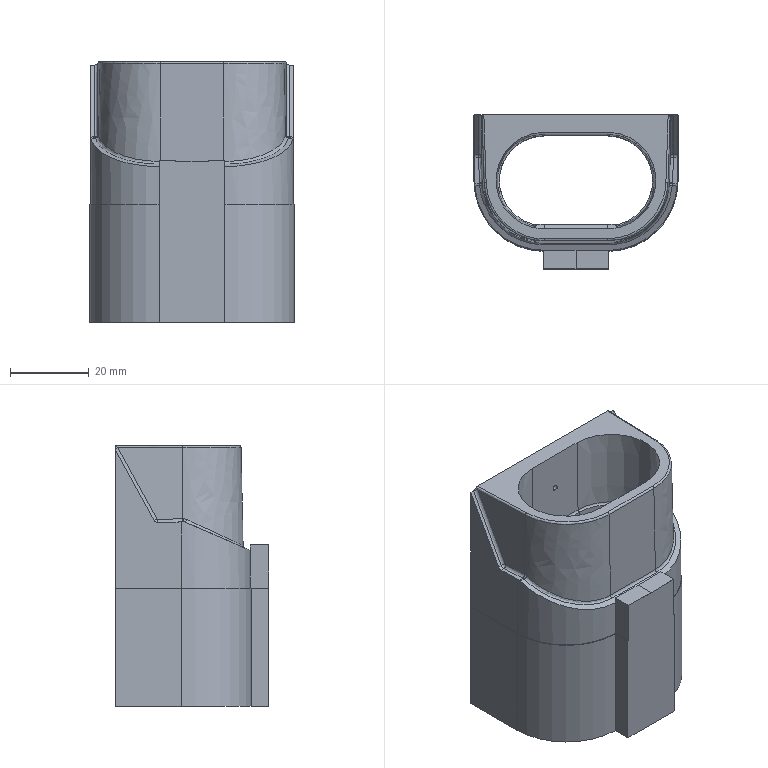Part | STEP file | lll_id82_x_t | 1 solid | 81 faces | box 51.763 x 39.033 x 66.18 mm | volume 54885 mm3 | plane 28 | spline 28 | cylinder 18 | torus 4 | cone 3 | commonest cylinder face diameters 2.008 x4 35.14 x4 0.602 x2 1.004 x2 22.83 x2 35.54 x2